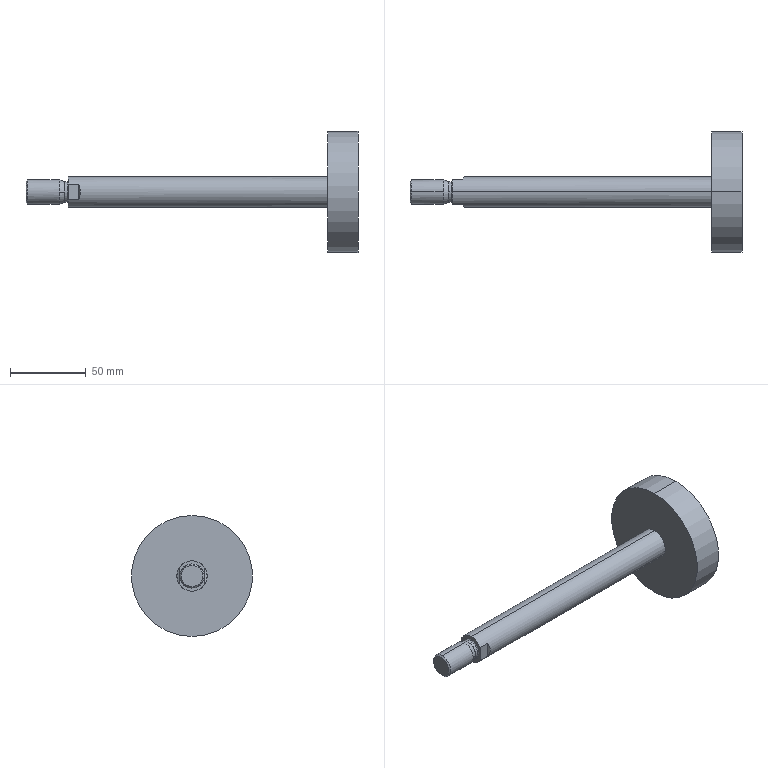Part | SolidWorks | features BaseBody 1 | 1 solid | 24 faces | box 219.5 x 80 x 80 mm | volume 159613 mm3 | cylinder 8 | plane 8 | spline 4 | cone 4 | commonest cylinder face diameters 13.5 x2 16 x2 20 x2 80 x2
STEP:
#1=CARTESIAN_POINT('',(-9.65,0.,6.75));
#2=VERTEX_POINT('',#1);
#3=CARTESIAN_POINT('',(-9.65,0.,-6.75));
#4=VERTEX_POINT('',#3);
#5=CARTESIAN_POINT('',(-9.65,0.,0.));
#6=DIRECTION('',(-1.,0.,0.));
#7=DIRECTION('',(0.,0.,-1.));
#8=AXIS2_PLACEMENT_3D('',#5,#6,#7);
#9=CIRCLE('',#8,6.75);
#10=EDGE_CURVE('',#2,#4,#9,.T.);
#11=ORIENTED_EDGE('',*,*,#10,.F.);
#12=CARTESIAN_POINT('',(-8.9,0.,7.5));
#13=VERTEX_POINT('',#12);
#14=CARTESIAN_POINT('',(-9.65,0.,7.5));
#15=DIRECTION('',(0.,-1.,0.));
#16=DIRECTION('',(0.,0.,1.));
#17=AXIS2_PLACEMENT_3D('',#14,#15,#16);
#18=CIRCLE('',#17,0.75);
#19=EDGE_CURVE('',#2,#13,#18,.T.);
#20=ORIENTED_EDGE('',*,*,#19,.T.);
#21=CARTESIAN_POINT('',(-8.9,0.,-7.5));
#22=VERTEX_POINT('',#21);
#23=CARTESIAN_POINT('',(-8.9,0.,7.5));
#24=CARTESIAN_POINT('',(-8.9,15.,7.5));
#25=CARTESIAN_POINT('',(-8.9,15.,-7.5));
#26=CARTESIAN_POINT('',(-8.9,0.,-7.5));
#27=(BOUNDED_CURVE()B_SPLINE_CURVE(3,(#23,#24,#25,#26),.UNSPECIFIED.,.F.,.T.)B_SPLINE_CURVE_WITH_KNOTS((4,4),(0.5,1.),.UNSPECIFIED.)CURVE()GEOMETRIC_REPRESENTATION_ITEM()RATIONAL_B_SPLINE_CURVE((1.,0.3333,0.3333,1.))REPRESENTATION_ITEM(''));
#28=EDGE_CURVE('',#13,#22,#27,.T.);
#29=ORIENTED_EDGE('',*,*,#28,.T.);
#30=CARTESIAN_POINT('',(-9.65,0.,-7.5));
#31=DIRECTION('',(0.,1.,0.));
#32=DIRECTION('',(0.,0.,-1.));
#33=AXIS2_PLACEMENT_3D('',#30,#31,#32);
#34=CIRCLE('',#33,0.75);
#35=EDGE_CURVE('',#4,#22,#34,.T.);
#36=ORIENTED_EDGE('',*,*,#35,.F.);
#37=EDGE_LOOP('',(#11,#20,#29,#36));
#38=FACE_OUTER_BOUND('',#37,.T.);
#39=CARTESIAN_POINT('',(-9.65,0.,-6.75));
#40=CARTESIAN_POINT('',(-9.65,13.5,-6.75));
#41=CARTESIAN_POINT('',(-9.65,13.5,6.75));
#42=CARTESIAN_POINT('',(-9.65,0.,6.75));
#43=CARTESIAN_POINT('',(-9.211,0.,-6.75));
#44=CARTESIAN_POINT('',(-9.211,13.5,-6.75));
#45=CARTESIAN_POINT('',(-9.211,13.5,6.75));
#46=CARTESIAN_POINT('',(-9.211,0.,6.75));
#47=CARTESIAN_POINT('',(-8.9,0.,-7.061));
#48=CARTESIAN_POINT('',(-8.9,14.121,-7.061));
#49=CARTESIAN_POINT('',(-8.9,14.121,7.061));
#50=CARTESIAN_POINT('',(-8.9,0.,7.061));
#51=CARTESIAN_POINT('',(-8.9,0.,-7.5));
#52=CARTESIAN_POINT('',(-8.9,15.,-7.5));
#53=CARTESIAN_POINT('',(-8.9,15.,7.5));
#54=CARTESIAN_POINT('',(-8.9,0.,7.5));
#55=(BOUNDED_SURFACE()B_SPLINE_SURFACE(3,3,((#39,#40,#41,#42),(#43,#44,#45,#46),(#47,#48,#49,#50),(#51,#52,#53,#54)),.UNSPECIFIED.,.F.,.F.,.T.)B_SPLINE_SURFACE_WITH_KNOTS((4,4),(4,4),(0.,1.),(0.,1.),.UNSPECIFIED.)GEOMETRIC_REPRESENTATION_ITEM()RATIONAL_B_SPLINE_SURFACE(((1.,0.3333,0.3333,1.),(0.8047,0.2682,0.2682,0.8047),(0.8047,0.2682,0.2682,0.8047),(1.,0.3333,0.3333,1.)))REPRESENTATION_ITEM('')SURFACE());
#56=ADVANCED_FACE('',(#38),#55,.F.);
#57=CARTESIAN_POINT('',(-11.624,0.,6.795));
#58=VERTEX_POINT('',#57);
#59=CARTESIAN_POINT('',(-11.624,6.795,0.));
#60=VERTEX_POINT('',#59);
#61=CARTESIAN_POINT('',(-11.624,0.,0.));
#62=DIRECTION('',(-1.,0.,0.));
#63=DIRECTION('',(0.,0.,-1.));
#64=AXIS2_PLACEMENT_3D('',#61,#62,#63);
#65=CIRCLE('',#64,6.795);
#66=EDGE_CURVE('',#58,#60,#65,.T.);
#67=ORIENTED_EDGE('',*,*,#66,.F.);
#68=CARTESIAN_POINT('',(-11.368,0.,6.75));
#69=VERTEX_POINT('',#68);
#70=CARTESIAN_POINT('',(-11.368,0.,7.5));
#71=DIRECTION('',(0.,-1.,0.));
#72=DIRECTION('',(0.,0.,1.));
#73=AXIS2_PLACEMENT_3D('',#70,#71,#72);
#74=CIRCLE('',#73,0.75);
#75=EDGE_CURVE('',#58,#69,#74,.T.);
#76=ORIENTED_EDGE('',*,*,#75,.T.);
#77=CARTESIAN_POINT('',(-11.368,0.,-6.75));
#78=VERTEX_POINT('',#77);
#79=CARTESIAN_POINT('',(-11.368,0.,0.));
#80=DIRECTION('',(1.,0.,0.));
#81=DIRECTION('',(0.,0.,1.));
#82=AXIS2_PLACEMENT_3D('',#79,#80,#81);
#83=CIRCLE('',#82,6.75);
#84=EDGE_CURVE('',#78,#69,#83,.T.);
#85=ORIENTED_EDGE('',*,*,#84,.F.);
#86=CARTESIAN_POINT('',(-11.624,0.,-6.795));
#87=VERTEX_POINT('',#86);
#88=CARTESIAN_POINT('',(-11.368,0.,-7.5));
#89=DIRECTION('',(0.,1.,0.));
#90=DIRECTION('',(0.,0.,-1.));
#91=AXIS2_PLACEMENT_3D('',#88,#89,#90);
#92=CIRCLE('',#91,0.75);
#93=EDGE_CURVE('',#87,#78,#92,.T.);
#94=ORIENTED_EDGE('',*,*,#93,.F.);
#95=CARTESIAN_POINT('',(-11.624,0.,0.));
#96=DIRECTION('',(-1.,0.,0.));
#97=DIRECTION('',(0.,0.,-1.));
#98=AXIS2_PLACEMENT_3D('',#95,#96,#97);
#99=CIRCLE('',#98,6.795);
#100=EDGE_CURVE('',#60,#87,#99,.T.);
#101=ORIENTED_EDGE('',*,*,#100,.F.);
#102=EDGE_LOOP('',(#67,#76,#85,#94,#101));
#103=FACE_OUTER_BOUND('',#102,.T.);
#104=CARTESIAN_POINT('',(-11.624,0.,-6.795));
#105=CARTESIAN_POINT('',(-11.624,13.59,-6.795));
#106=CARTESIAN_POINT('',(-11.624,13.59,6.795));
#107=CARTESIAN_POINT('',(-11.624,0.,6.795));
#108=CARTESIAN_POINT('',(-11.542,0.,-6.765));
#109=CARTESIAN_POINT('',(-11.542,13.53,-6.765));
#110=CARTESIAN_POINT('',(-11.542,13.53,6.765));
#111=CARTESIAN_POINT('',(-11.542,0.,6.765));
#112=CARTESIAN_POINT('',(-11.455,0.,-6.75));
#113=CARTESIAN_POINT('',(-11.455,13.5,-6.75));
#114=CARTESIAN_POINT('',(-11.455,13.5,6.75));
#115=CARTESIAN_POINT('',(-11.455,0.,6.75));
#116=CARTESIAN_POINT('',(-11.368,0.,-6.75));
#117=CARTESIAN_POINT('',(-11.368,13.5,-6.75));
#118=CARTESIAN_POINT('',(-11.368,13.5,6.75));
#119=CARTESIAN_POINT('',(-11.368,0.,6.75));
#120=(BOUNDED_SURFACE()B_SPLINE_SURFACE(3,3,((#104,#105,#106,#107),(#108,#109,#110,#111),(#112,#113,#114,#115),(#116,#117,#118,#119)),.UNSPECIFIED.,.F.,.F.,.F.)B_SPLINE_SURFACE_WITH_KNOTS((4,4),(4,4),(0.,1.),(0.,1.),.UNSPECIFIED.)GEOMETRIC_REPRESENTATION_ITEM()RATIONAL_B_SPLINE_SURFACE(((1.,0.3333,0.3333,1.),(0.9899,0.33,0.33,0.9899),(0.9899,0.33,0.33,0.9899),(1.,0.3333,0.3333,1.)))REPRESENTATION_ITEM('')SURFACE());
#121=ADVANCED_FACE('',(#103),#120,.F.);
#122=CARTESIAN_POINT('',(162.6,0.,10.));
#123=VERTEX_POINT('',#122);
#124=CARTESIAN_POINT('',(162.6,0.,-10.));
#125=VERTEX_POINT('',#124);
#126=CARTESIAN_POINT('',(162.6,0.,0.));
#127=DIRECTION('',(-1.,0.,0.));
#128=DIRECTION('',(0.,0.,1.));
#129=AXIS2_PLACEMENT_3D('',#126,#127,#128);
#130=CIRCLE('',#129,10.);
#131=EDGE_CURVE('',#123,#125,#130,.T.);
#132=ORIENTED_EDGE('',*,*,#131,.T.);
#133=CARTESIAN_POINT('',(-8.9,0.,-10.));
#134=VERTEX_POINT('',#133);
#135=CARTESIAN_POINT('',(182.6,0.,-10.));
#136=DIRECTION('',(-1.,0.,0.));
#137=VECTOR('',#136,1000.);
#138=LINE('',#135,#137);
#139=EDGE_CURVE('',#125,#134,#138,.T.);
#140=ORIENTED_EDGE('',*,*,#139,.T.);
#141=CARTESIAN_POINT('',(-8.9,8.5,-5.268));
#142=VERTEX_POINT('',#141);
#143=CARTESIAN_POINT('',(-8.9,0.,0.));
#144=DIRECTION('',(1.,0.,0.));
#145=DIRECTION('',(0.,0.,1.));
#146=AXIS2_PLACEMENT_3D('',#143,#144,#145);
#147=CIRCLE('',#146,10.);
#148=EDGE_CURVE('',#134,#142,#147,.T.);
#149=ORIENTED_EDGE('',*,*,#148,.T.);
#150=CARTESIAN_POINT('',(-1.9,8.5,-5.268));
#151=VERTEX_POINT('',#150);
#152=CARTESIAN_POINT('',(182.6,8.5,-5.268));
#153=DIRECTION('',(1.,0.,0.));
#154=VECTOR('',#153,1000.);
#155=LINE('',#152,#154);
#156=EDGE_CURVE('',#142,#151,#155,.T.);
#157=ORIENTED_EDGE('',*,*,#156,.T.);
#158=CARTESIAN_POINT('',(-1.9,8.5,5.268));
#159=VERTEX_POINT('',#158);
#160=CARTESIAN_POINT('',(-1.9,8.5,-5.268));
#161=CARTESIAN_POINT('',(-0.7132,10.556,-1.951));
#162=CARTESIAN_POINT('',(-0.7132,10.556,1.951));
#163=CARTESIAN_POINT('',(-1.9,8.5,5.268));
#164=(BOUNDED_CURVE()B_SPLINE_CURVE(3,(#160,#161,#162,#163),.UNSPECIFIED.,.F.,.F.)B_SPLINE_CURVE_WITH_KNOTS((4,4),(2.587,3.696),.UNSPECIFIED.)CURVE()GEOMETRIC_REPRESENTATION_ITEM()RATIONAL_B_SPLINE_CURVE((1.,0.9,0.9,1.))REPRESENTATION_ITEM(''));
#165=EDGE_CURVE('',#151,#159,#164,.T.);
#166=ORIENTED_EDGE('',*,*,#165,.T.);
#167=CARTESIAN_POINT('',(-8.9,8.5,5.268));
#168=VERTEX_POINT('',#167);
#169=CARTESIAN_POINT('',(182.6,8.5,5.268));
#170=DIRECTION('',(-1.,0.,0.));
#171=VECTOR('',#170,1000.);
#172=LINE('',#169,#171);
#173=EDGE_CURVE('',#159,#168,#172,.T.);
#174=ORIENTED_EDGE('',*,*,#173,.T.);
#175=CARTESIAN_POINT('',(-8.9,0.,10.));
#176=VERTEX_POINT('',#175);
#177=CARTESIAN_POINT('',(-8.9,0.,0.));
#178=DIRECTION('',(1.,0.,0.));
#179=DIRECTION('',(0.,0.,1.));
#180=AXIS2_PLACEMENT_3D('',#177,#178,#179);
#181=CIRCLE('',#180,10.);
#182=EDGE_CURVE('',#168,#176,#181,.T.);
#183=ORIENTED_EDGE('',*,*,#182,.T.);
#184=CARTESIAN_POINT('',(182.6,0.,10.));
#185=DIRECTION('',(-1.,0.,0.));
#186=VECTOR('',#185,1000.);
#187=LINE('',#184,#186);
#188=EDGE_CURVE('',#123,#176,#187,.T.);
#189=ORIENTED_EDGE('',*,*,#188,.F.);
#190=EDGE_LOOP('',(#132,#140,#149,#157,#166,#174,#183,#189));
#191=FACE_OUTER_BOUND('',#190,.T.);
#192=CARTESIAN_POINT('',(182.6,0.,0.));
#193=DIRECTION('',(-1.,0.,0.));
#194=DIRECTION('',(0.,0.,1.));
#195=AXIS2_PLACEMENT_3D('',#192,#193,#194);
#196=CYLINDRICAL_SURFACE('',#195,10.);
#197=ADVANCED_FACE('',(#191),#196,.T.);
#198=CARTESIAN_POINT('',(182.6,0.,40.));
#199=VERTEX_POINT('',#198);
#200=CARTESIAN_POINT('',(182.6,0.,-40.));
#201=VERTEX_POINT('',#200);
#202=CARTESIAN_POINT('',(182.6,0.,0.));
#203=DIRECTION('',(-1.,0.,0.));
#204=DIRECTION('',(0.,0.,1.));
#205=AXIS2_PLACEMENT_3D('',#202,#203,#204);
#206=CIRCLE('',#205,40.);
#207=EDGE_CURVE('',#199,#201,#206,.T.);
#208=ORIENTED_EDGE('',*,*,#207,.T.);
#209=CARTESIAN_POINT('',(162.6,0.,-40.));
#210=VERTEX_POINT('',#209);
#211=CARTESIAN_POINT('',(182.6,0.,-40.));
#212=DIRECTION('',(-1.,0.,0.));
#213=VECTOR('',#212,1000.);
#214=LINE('',#211,#213);
#215=EDGE_CURVE('',#201,#210,#214,.T.);
#216=ORIENTED_EDGE('',*,*,#215,.T.);
#217=CARTESIAN_POINT('',(162.6,0.,40.));
#218=VERTEX_POINT('',#217);
#219=CARTESIAN_POINT('',(162.6,0.,0.));
#220=DIRECTION('',(1.,0.,0.));
#221=DIRECTION('',(0.,0.,1.));
#222=AXIS2_PLACEMENT_3D('',#219,#220,#221);
#223=CIRCLE('',#222,40.);
#224=EDGE_CURVE('',#210,#218,#223,.T.);
#225=ORIENTED_EDGE('',*,*,#224,.T.);
#226=CARTESIAN_POINT('',(182.6,0.,40.));
#227=DIRECTION('',(-1.,0.,0.));
#228=VECTOR('',#227,1000.);
#229=LINE('',#226,#228);
#230=EDGE_CURVE('',#199,#218,#229,.T.);
#231=ORIENTED_EDGE('',*,*,#230,.F.);
#232=EDGE_LOOP('',(#208,#216,#225,#231));
#233=FACE_OUTER_BOUND('',#232,.T.);
#234=CARTESIAN_POINT('',(182.6,0.,0.));
#235=DIRECTION('',(-1.,0.,0.));
#236=DIRECTION('',(0.,0.,1.));
#237=AXIS2_PLACEMENT_3D('',#234,#235,#236);
#238=CYLINDRICAL_SURFACE('',#237,40.);
#239=ADVANCED_FACE('',(#233),#238,.T.);
#240=ORIENTED_EDGE('',*,*,#10,.T.);
#241=CARTESIAN_POINT('',(-7.9,0.,-6.75));
#242=DIRECTION('',(-1.,0.,0.));
#243=VECTOR('',#242,1000.);
#244=LINE('',#241,#243);
#245=EDGE_CURVE('',#4,#78,#244,.T.);
#246=ORIENTED_EDGE('',*,*,#245,.T.);
#247=ORIENTED_EDGE('',*,*,#84,.T.);
#248=CARTESIAN_POINT('',(-7.9,0.,6.75));
#249=DIRECTION('',(-1.,0.,0.));
#250=VECTOR('',#249,1000.);
#251=LINE('',#248,#250);
#252=EDGE_CURVE('',#2,#69,#251,.T.);
#253=ORIENTED_EDGE('',*,*,#252,.F.);
#254=EDGE_LOOP('',(#240,#246,#247,#253));
#255=FACE_OUTER_BOUND('',#254,.T.);
#256=CARTESIAN_POINT('',(-7.9,0.,0.));
#257=DIRECTION('',(-1.,0.,0.));
#258=DIRECTION('',(0.,0.,1.));
#259=AXIS2_PLACEMENT_3D('',#256,#257,#258);
#260=CYLINDRICAL_SURFACE('',#259,6.75);
#261=ADVANCED_FACE('',(#255),#260,.T.);
#262=CARTESIAN_POINT('',(-11.624,-6.795,0.));
#263=VERTEX_POINT('',#262);
#264=CARTESIAN_POINT('',(-11.624,0.,0.));
#265=DIRECTION('',(-1.,0.,0.));
#266=DIRECTION('',(0.,0.,-1.));
#267=AXIS2_PLACEMENT_3D('',#264,#265,#266);
#268=CIRCLE('',#267,6.795);
#269=EDGE_CURVE('',#263,#58,#268,.T.);
#270=ORIENTED_EDGE('',*,*,#269,.T.);
#271=ORIENTED_EDGE('',*,*,#66,.T.);
#272=CARTESIAN_POINT('',(-14.934,8.,0.));
#273=VERTEX_POINT('',#272);
#274=CARTESIAN_POINT('',(-14.934,8.,0.));
#275=DIRECTION('',(-0.9397,0.342,0.));
#276=VECTOR('',#275,1000.);
#277=LINE('',#274,#276);
#278=EDGE_CURVE('',#60,#273,#277,.T.);
#279=ORIENTED_EDGE('',*,*,#278,.T.);
#280=CARTESIAN_POINT('',(-14.934,0.,8.));
#281=VERTEX_POINT('',#280);
#282=CARTESIAN_POINT('',(-14.934,0.,0.));
#283=DIRECTION('',(1.,0.,0.));
#284=DIRECTION('',(0.,0.,1.));
#285=AXIS2_PLACEMENT_3D('',#282,#283,#284);
#286=CIRCLE('',#285,8.);
#287=EDGE_CURVE('',#273,#281,#286,.T.);
#288=ORIENTED_EDGE('',*,*,#287,.T.);
#289=CARTESIAN_POINT('',(-14.934,-8.,0.));
#290=VERTEX_POINT('',#289);
#291=CARTESIAN_POINT('',(-14.934,0.,0.));
#292=DIRECTION('',(1.,0.,0.));
#293=DIRECTION('',(0.,0.,1.));
#294=AXIS2_PLACEMENT_3D('',#291,#292,#293);
#295=CIRCLE('',#294,8.);
#296=EDGE_CURVE('',#281,#290,#295,.T.);
#297=ORIENTED_EDGE('',*,*,#296,.T.);
#298=CARTESIAN_POINT('',(-14.934,-8.,0.));
#299=DIRECTION('',(-0.9397,-0.342,0.));
#300=VECTOR('',#299,1000.);
#301=LINE('',#298,#300);
#302=EDGE_CURVE('',#263,#290,#301,.T.);
#303=ORIENTED_EDGE('',*,*,#302,.F.);
#304=EDGE_LOOP('',(#270,#271,#279,#288,#297,#303));
#305=FACE_OUTER_BOUND('',#304,.T.);
#306=CARTESIAN_POINT('',(-14.934,0.,0.));
#307=DIRECTION('',(-1.,0.,0.));
#308=DIRECTION('',(0.,-1.,0.));
#309=AXIS2_PLACEMENT_3D('',#306,#307,#308);
#310=CONICAL_SURFACE('',#309,8.,0.3491);
#311=ADVANCED_FACE('',(#305),#310,.T.);
#312=CARTESIAN_POINT('',(-14.934,0.,-8.));
#313=VERTEX_POINT('',#312);
#314=CARTESIAN_POINT('',(-14.934,0.,0.));
#315=DIRECTION('',(1.,0.,0.));
#316=DIRECTION('',(0.,0.,1.));
#317=AXIS2_PLACEMENT_3D('',#314,#315,#316);
#318=CIRCLE('',#317,8.);
#319=EDGE_CURVE('',#313,#273,#318,.T.);
#320=ORIENTED_EDGE('',*,*,#319,.F.);
#321=CARTESIAN_POINT('',(-35.98,0.,-8.));
#322=VERTEX_POINT('',#321);
#323=CARTESIAN_POINT('',(-7.9,0.,-8.));
#324=DIRECTION('',(-1.,0.,0.));
#325=VECTOR('',#324,1000.);
#326=LINE('',#323,#325);
#327=EDGE_CURVE('',#313,#322,#326,.T.);
#328=ORIENTED_EDGE('',*,*,#327,.T.);
#329=CARTESIAN_POINT('',(-35.98,0.,8.));
#330=VERTEX_POINT('',#329);
#331=CARTESIAN_POINT('',(-35.98,0.,0.));
#332=DIRECTION('',(1.,0.,0.));
#333=DIRECTION('',(0.,0.,1.));
#334=AXIS2_PLACEMENT_3D('',#331,#332,#333);
#335=CIRCLE('',#334,8.);
#336=EDGE_CURVE('',#322,#330,#335,.T.);
#337=ORIENTED_EDGE('',*,*,#336,.T.);
#338=CARTESIAN_POINT('',(-7.9,0.,8.));
#339=DIRECTION('',(-1.,0.,0.));
#340=VECTOR('',#339,1000.);
#341=LINE('',#338,#340);
#342=EDGE_CURVE('',#281,#330,#341,.T.);
#343=ORIENTED_EDGE('',*,*,#342,.F.);
#344=ORIENTED_EDGE('',*,*,#287,.F.);
#345=EDGE_LOOP('',(#320,#328,#337,#343,#344));
#346=FACE_OUTER_BOUND('',#345,.T.);
#347=CARTESIAN_POINT('',(-7.9,0.,0.));
#348=DIRECTION('',(-1.,0.,0.));
#349=DIRECTION('',(0.,0.,1.));
#350=AXIS2_PLACEMENT_3D('',#347,#348,#349);
#351=CYLINDRICAL_SURFACE('',#350,8.);
#352=ADVANCED_FACE('',(#346),#351,.T.);
#353=CARTESIAN_POINT('',(-36.9,0.,-7.08));
#354=VERTEX_POINT('',#353);
#355=CARTESIAN_POINT('',(-36.9,0.,7.08));
#356=VERTEX_POINT('',#355);
#357=CARTESIAN_POINT('',(-36.9,0.,0.));
#358=DIRECTION('',(1.,0.,0.));
#359=DIRECTION('',(0.,0.,-1.));
#360=AXIS2_PLACEMENT_3D('',#357,#358,#359);
#361=CIRCLE('',#360,7.08);
#362=EDGE_CURVE('',#354,#356,#361,.T.);
#363=ORIENTED_EDGE('',*,*,#362,.T.);
#364=CARTESIAN_POINT('',(-35.98,0.,8.));
#365=DIRECTION('',(0.7071,0.,0.7071));
#366=VECTOR('',#365,1000.);
#367=LINE('',#364,#366);
#368=EDGE_CURVE('',#356,#330,#367,.T.);
#369=ORIENTED_EDGE('',*,*,#368,.T.);
#370=ORIENTED_EDGE('',*,*,#336,.F.);
#371=CARTESIAN_POINT('',(-35.98,0.,-8.));
#372=DIRECTION('',(0.7071,0.,-0.7071));
#373=VECTOR('',#372,1000.);
#374=LINE('',#371,#373);
#375=EDGE_CURVE('',#354,#322,#374,.T.);
#376=ORIENTED_EDGE('',*,*,#375,.F.);
#377=EDGE_LOOP('',(#363,#369,#370,#376));
#378=FACE_OUTER_BOUND('',#377,.T.);
#379=CARTESIAN_POINT('',(-35.98,0.,0.));
#380=DIRECTION('',(1.,0.,0.));
#381=DIRECTION('',(0.,0.,-1.));
#382=AXIS2_PLACEMENT_3D('',#379,#380,#381);
#383=CONICAL_SURFACE('',#382,8.,0.7854);
#384=ADVANCED_FACE('',(#378),#383,.T.);
#385=ORIENTED_EDGE('',*,*,#139,.F.);
#386=CARTESIAN_POINT('',(162.6,0.,0.));
#387=DIRECTION('',(-1.,0.,0.));
#388=DIRECTION('',(0.,0.,1.));
#389=AXIS2_PLACEMENT_3D('',#386,#387,#388);
#390=CIRCLE('',#389,10.);
#391=EDGE_CURVE('',#125,#123,#390,.T.);
#392=ORIENTED_EDGE('',*,*,#391,.T.);
#393=ORIENTED_EDGE('',*,*,#188,.T.);
#394=CARTESIAN_POINT('',(-8.9,-8.5,5.268));
#395=VERTEX_POINT('',#394);
#396=CARTESIAN_POINT('',(-8.9,0.,0.));
#397=DIRECTION('',(1.,0.,0.));
#398=DIRECTION('',(0.,0.,1.));
#399=AXIS2_PLACEMENT_3D('',#396,#397,#398);
#400=CIRCLE('',#399,10.);
#401=EDGE_CURVE('',#176,#395,#400,.T.);
#402=ORIENTED_EDGE('',*,*,#401,.T.);
#403=CARTESIAN_POINT('',(-1.9,-8.5,5.268));
#404=VERTEX_POINT('',#403);
#405=CARTESIAN_POINT('',(182.6,-8.5,5.268));
#406=DIRECTION('',(1.,0.,0.));
#407=VECTOR('',#406,1000.);
#408=LINE('',#405,#407);
#409=EDGE_CURVE('',#395,#404,#408,.T.);
#410=ORIENTED_EDGE('',*,*,#409,.T.);
#411=CARTESIAN_POINT('',(-1.9,-8.5,-5.268));
#412=VERTEX_POINT('',#411);
#413=CARTESIAN_POINT('',(-1.9,-8.5,5.268));
#414=CARTESIAN_POINT('',(-0.7132,-10.556,1.951));
#415=CARTESIAN_POINT('',(-0.7132,-10.556,-1.951));
#416=CARTESIAN_POINT('',(-1.9,-8.5,-5.268));
#417=(BOUNDED_CURVE()B_SPLINE_CURVE(3,(#413,#414,#415,#416),.UNSPECIFIED.,.F.,.T.)B_SPLINE_CURVE_WITH_KNOTS((4,4),(2.587,3.696),.UNSPECIFIED.)CURVE()GEOMETRIC_REPRESENTATION_ITEM()RATIONAL_B_SPLINE_CURVE((1.,0.9,0.9,1.))REPRESENTATION_ITEM(''));
#418=EDGE_CURVE('',#404,#412,#417,.T.);
#419=ORIENTED_EDGE('',*,*,#418,.T.);
#420=CARTESIAN_POINT('',(-8.9,-8.5,-5.268));
#421=VERTEX_POINT('',#420);
#422=CARTESIAN_POINT('',(182.6,-8.5,-5.268));
#423=DIRECTION('',(-1.,0.,0.));
#424=VECTOR('',#423,1000.);
#425=LINE('',#422,#424);
#426=EDGE_CURVE('',#412,#421,#425,.T.);
#427=ORIENTED_EDGE('',*,*,#426,.T.);
#428=CARTESIAN_POINT('',(-8.9,0.,0.));
#429=DIRECTION('',(1.,0.,0.));
#430=DIRECTION('',(0.,0.,1.));
#431=AXIS2_PLACEMENT_3D('',#428,#429,#430);
#432=CIRCLE('',#431,10.);
#433=EDGE_CURVE('',#421,#134,#432,.T.);
#434=ORIENTED_EDGE('',*,*,#433,.T.);
#435=EDGE_LOOP('',(#385,#392,#393,#402,#410,#419,#427,#434));
#436=FACE_OUTER_BOUND('',#435,.T.);
#437=CARTESIAN_POINT('',(182.6,0.,0.));
#438=DIRECTION('',(-1.,0.,0.));
#439=DIRECTION('',(0.,0.,1.));
#440=AXIS2_PLACEMENT_3D('',#437,#438,#439);
#441=CYLINDRICAL_SURFACE('',#440,10.);
#442=ADVANCED_FACE('',(#436),#441,.T.);
#443=ORIENTED_EDGE('',*,*,#418,.F.);
#444=CARTESIAN_POINT('',(-1.9,-8.5,20.));
#445=DIRECTION('',(0.,0.,-1.));
#446=VECTOR('',#445,1000.);
#447=LINE('',#444,#446);
#448=EDGE_CURVE('',#404,#412,#447,.T.);
#449=ORIENTED_EDGE('',*,*,#448,.T.);
#450=EDGE_LOOP('',(#443,#449));
#451=FACE_OUTER_BOUND('',#450,.T.);
#452=CARTESIAN_POINT('',(6.76,-23.5,20.));
#453=DIRECTION('',(-0.866,-0.5,0.));
#454=DIRECTION('',(0.5,-0.866,0.));
#455=AXIS2_PLACEMENT_3D('',#452,#453,#454);
#456=PLANE('',#455);
#457=ADVANCED_FACE('',(#451),#456,.T.);
#458=ORIENTED_EDGE('',*,*,#409,.F.);
#459=CARTESIAN_POINT('',(-8.9,-8.5,20.));
#460=DIRECTION('',(0.,0.,-1.));
#461=VECTOR('',#460,1000.);
#462=LINE('',#459,#461);
#463=EDGE_CURVE('',#395,#421,#462,.T.);
#464=ORIENTED_EDGE('',*,*,#463,.T.);
#465=ORIENTED_EDGE('',*,*,#426,.F.);
#466=ORIENTED_EDGE('',*,*,#448,.F.);
#467=EDGE_LOOP('',(#458,#464,#465,#466));
#468=FACE_OUTER_BOUND('',#467,.T.);
#469=CARTESIAN_POINT('',(-1.9,-8.5,20.));
#470=DIRECTION('',(0.,-1.,0.));
#471=DIRECTION('',(0.,0.,-1.));
#472=AXIS2_PLACEMENT_3D('',#469,#470,#471);
#473=PLANE('',#472);
#474=ADVANCED_FACE('',(#468),#473,.T.);
#475=CARTESIAN_POINT('',(-8.9,0.,-7.5));
#476=CARTESIAN_POINT('',(-8.9,-15.,-7.5));
#477=CARTESIAN_POINT('',(-8.9,-15.,7.5));
#478=CARTESIAN_POINT('',(-8.9,0.,7.5));
#479=(BOUNDED_CURVE()B_SPLINE_CURVE(3,(#475,#476,#477,#478),.UNSPECIFIED.,.F.,.T.)B_SPLINE_CURVE_WITH_KNOTS((4,4),(0.,0.5),.UNSPECIFIED.)CURVE()GEOMETRIC_REPRESENTATION_ITEM()RATIONAL_B_SPLINE_CURVE((1.,0.3333,0.3333,1.))REPRESENTATION_ITEM(''));
#480=EDGE_CURVE('',#22,#13,#479,.T.);
#481=ORIENTED_EDGE('',*,*,#480,.F.);
#482=ORIENTED_EDGE('',*,*,#28,.F.);
#483=EDGE_LOOP('',(#481,#482));
#484=FACE_BOUND('',#483,.T.);
#485=ORIENTED_EDGE('',*,*,#433,.F.);
#486=ORIENTED_EDGE('',*,*,#463,.F.);
#487=ORIENTED_EDGE('',*,*,#401,.F.);
#488=ORIENTED_EDGE('',*,*,#182,.F.);
#489=CARTESIAN_POINT('',(-8.9,8.5,0.));
#490=DIRECTION('',(0.,0.,1.));
#491=VECTOR('',#490,1000.);
#492=LINE('',#489,#491);
#493=EDGE_CURVE('',#142,#168,#492,.T.);
#494=ORIENTED_EDGE('',*,*,#493,.F.);
#495=ORIENTED_EDGE('',*,*,#148,.F.);
#496=EDGE_LOOP('',(#485,#486,#487,#488,#494,#495));
#497=FACE_OUTER_BOUND('',#496,.T.);
#498=CARTESIAN_POINT('',(-8.9,0.,0.));
#499=DIRECTION('',(1.,0.,0.));
#500=DIRECTION('',(0.,0.,-1.));
#501=AXIS2_PLACEMENT_3D('',#498,#499,#500);
#502=PLANE('',#501);
#503=ADVANCED_FACE('',(#484,#497),#502,.F.);
#504=ORIENTED_EDGE('',*,*,#156,.F.);
#505=ORIENTED_EDGE('',*,*,#493,.T.);
#506=ORIENTED_EDGE('',*,*,#173,.F.);
#507=CARTESIAN_POINT('',(-1.9,8.5,20.));
#508=DIRECTION('',(0.,0.,-1.));
#509=VECTOR('',#508,1000.);
#510=LINE('',#507,#509);
#511=EDGE_CURVE('',#159,#151,#510,.T.);
#512=ORIENTED_EDGE('',*,*,#511,.T.);
#513=EDGE_LOOP('',(#504,#505,#506,#512));
#514=FACE_OUTER_BOUND('',#513,.T.);
#515=CARTESIAN_POINT('',(-8.9,8.5,20.));
#516=DIRECTION('',(0.,1.,0.));
#517=DIRECTION('',(0.,0.,1.));
#518=AXIS2_PLACEMENT_3D('',#515,#516,#517);
#519=PLANE('',#518);
#520=ADVANCED_FACE('',(#514),#519,.T.);
#521=ORIENTED_EDGE('',*,*,#165,.F.);
#522=ORIENTED_EDGE('',*,*,#511,.F.);
#523=EDGE_LOOP('',(#521,#522));
#524=FACE_OUTER_BOUND('',#523,.T.);
#525=CARTESIAN_POINT('',(-1.9,8.5,20.));
#526=DIRECTION('',(-0.866,0.5,0.));
#527=DIRECTION('',(-0.5,-0.866,0.));
#528=AXIS2_PLACEMENT_3D('',#525,#526,#527);
#529=PLANE('',#528);
#530=ADVANCED_FACE('',(#524),#529,.T.);
#531=ORIENTED_EDGE('',*,*,#131,.F.);
#532=ORIENTED_EDGE('',*,*,#391,.F.);
#533=EDGE_LOOP('',(#531,#532));
#534=FACE_BOUND('',#533,.T.);
#535=CARTESIAN_POINT('',(162.6,0.,0.));
#536=DIRECTION('',(1.,0.,0.));
#537=DIRECTION('',(0.,0.,1.));
#538=AXIS2_PLACEMENT_3D('',#535,#536,#537);
#539=CIRCLE('',#538,40.);
#540=EDGE_CURVE('',#218,#210,#539,.T.);
#541=ORIENTED_EDGE('',*,*,#540,.F.);
#542=ORIENTED_EDGE('',*,*,#224,.F.);
#543=EDGE_LOOP('',(#541,#542));
#544=FACE_OUTER_BOUND('',#543,.T.);
#545=CARTESIAN_POINT('',(162.6,0.,0.));
#546=DIRECTION('',(1.,0.,0.));
#547=DIRECTION('',(0.,0.,-1.));
#548=AXIS2_PLACEMENT_3D('',#545,#546,#547);
#549=PLANE('',#548);
#550=ADVANCED_FACE('',(#534,#544),#549,.F.);
#551=ORIENTED_EDGE('',*,*,#19,.F.);
#552=CARTESIAN_POINT('',(-9.65,0.,0.));
#553=DIRECTION('',(-1.,0.,0.));
#554=DIRECTION('',(0.,0.,-1.));
#555=AXIS2_PLACEMENT_3D('',#552,#553,#554);
#556=CIRCLE('',#555,6.75);
#557=EDGE_CURVE('',#4,#2,#556,.T.);
#558=ORIENTED_EDGE('',*,*,#557,.F.);
#559=ORIENTED_EDGE('',*,*,#35,.T.);
#560=ORIENTED_EDGE('',*,*,#480,.T.);
#561=EDGE_LOOP('',(#551,#558,#559,#560));
#562=FACE_OUTER_BOUND('',#561,.T.);
#563=CARTESIAN_POINT('',(-9.65,0.,6.75));
#564=CARTESIAN_POINT('',(-9.65,-13.5,6.75));
#565=CARTESIAN_POINT('',(-9.65,-13.5,-6.75));
#566=CARTESIAN_POINT('',(-9.65,0.,-6.75));
#567=CARTESIAN_POINT('',(-9.211,0.,6.75));
#568=CARTESIAN_POINT('',(-9.211,-13.5,6.75));
#569=CARTESIAN_POINT('',(-9.211,-13.5,-6.75));
#570=CARTESIAN_POINT('',(-9.211,0.,-6.75));
#571=CARTESIAN_POINT('',(-8.9,0.,7.061));
#572=CARTESIAN_POINT('',(-8.9,-14.121,7.061));
#573=CARTESIAN_POINT('',(-8.9,-14.121,-7.061));
#574=CARTESIAN_POINT('',(-8.9,0.,-7.061));
#575=CARTESIAN_POINT('',(-8.9,0.,7.5));
#576=CARTESIAN_POINT('',(-8.9,-15.,7.5));
#577=CARTESIAN_POINT('',(-8.9,-15.,-7.5));
#578=CARTESIAN_POINT('',(-8.9,0.,-7.5));
#579=(BOUNDED_SURFACE()B_SPLINE_SURFACE(3,3,((#563,#564,#565,#566),(#567,#568,#569,#570),(#571,#572,#573,#574),(#575,#576,#577,#578)),.UNSPECIFIED.,.F.,.F.,.F.)B_SPLINE_SURFACE_WITH_KNOTS((4,4),(4,4),(0.,1.),(0.,1.),.UNSPECIFIED.)GEOMETRIC_REPRESENTATION_ITEM()RATIONAL_B_SPLINE_SURFACE(((1.,0.3333,0.3333,1.),(0.8047,0.2682,0.2682,0.8047),(0.8047,0.2682,0.2682,0.8047),(1.,0.3333,0.3333,1.)))REPRESENTATION_ITEM('')SURFACE());
#580=ADVANCED_FACE('',(#562),#579,.F.);
#581=ORIENTED_EDGE('',*,*,#215,.F.);
#582=CARTESIAN_POINT('',(182.6,0.,0.));
#583=DIRECTION('',(-1.,0.,0.));
#584=DIRECTION('',(0.,0.,1.));
#585=AXIS2_PLACEMENT_3D('',#582,#583,#584);
#586=CIRCLE('',#585,40.);
#587=EDGE_CURVE('',#201,#199,#586,.T.);
#588=ORIENTED_EDGE('',*,*,#587,.T.);
#589=ORIENTED_EDGE('',*,*,#230,.T.);
#590=ORIENTED_EDGE('',*,*,#540,.T.);
#591=EDGE_LOOP('',(#581,#588,#589,#590));
#592=FACE_OUTER_BOUND('',#591,.T.);
#593=CARTESIAN_POINT('',(182.6,0.,0.));
#594=DIRECTION('',(-1.,0.,0.));
#595=DIRECTION('',(0.,0.,1.));
#596=AXIS2_PLACEMENT_3D('',#593,#594,#595);
#597=CYLINDRICAL_SURFACE('',#596,40.);
#598=ADVANCED_FACE('',(#592),#597,.T.);
#599=ORIENTED_EDGE('',*,*,#245,.F.);
#600=ORIENTED_EDGE('',*,*,#557,.T.);
#601=ORIENTED_EDGE('',*,*,#252,.T.);
#602=CARTESIAN_POINT('',(-11.368,0.,0.));
#603=DIRECTION('',(1.,0.,0.));
#604=DIRECTION('',(0.,0.,1.));
#605=AXIS2_PLACEMENT_3D('',#602,#603,#604);
#606=CIRCLE('',#605,6.75);
#607=EDGE_CURVE('',#69,#78,#606,.T.);
#608=ORIENTED_EDGE('',*,*,#607,.T.);
#609=EDGE_LOOP('',(#599,#600,#601,#608));
#610=FACE_OUTER_BOUND('',#609,.T.);
#611=CARTESIAN_POINT('',(-7.9,0.,0.));
#612=DIRECTION('',(-1.,0.,0.));
#613=DIRECTION('',(0.,0.,1.));
#614=AXIS2_PLACEMENT_3D('',#611,#612,#613);
#615=CYLINDRICAL_SURFACE('',#614,6.75);
#616=ADVANCED_FACE('',(#610),#615,.T.);
#617=ORIENTED_EDGE('',*,*,#207,.F.);
#618=ORIENTED_EDGE('',*,*,#587,.F.);
#619=EDGE_LOOP('',(#617,#618));
#620=FACE_OUTER_BOUND('',#619,.T.);
#621=CARTESIAN_POINT('',(182.6,10.,0.));
#622=DIRECTION('',(-1.,0.,0.));
#623=DIRECTION('',(0.,0.,1.));
#624=AXIS2_PLACEMENT_3D('',#621,#622,#623);
#625=PLANE('',#624);
#626=ADVANCED_FACE('',(#620),#625,.F.);
#627=ORIENTED_EDGE('',*,*,#75,.F.);
#628=ORIENTED_EDGE('',*,*,#269,.F.);
#629=CARTESIAN_POINT('',(-11.624,0.,0.));
#630=DIRECTION('',(-1.,0.,0.));
#631=DIRECTION('',(0.,0.,-1.));
#632=AXIS2_PLACEMENT_3D('',#629,#630,#631);
#633=CIRCLE('',#632,6.795);
#634=EDGE_CURVE('',#87,#263,#633,.T.);
#635=ORIENTED_EDGE('',*,*,#634,.F.);
#636=ORIENTED_EDGE('',*,*,#93,.T.);
#637=ORIENTED_EDGE('',*,*,#607,.F.);
#638=EDGE_LOOP('',(#627,#628,#635,#636,#637));
#639=FACE_OUTER_BOUND('',#638,.T.);
#640=CARTESIAN_POINT('',(-11.624,0.,6.795));
#641=CARTESIAN_POINT('',(-11.624,-13.59,6.795));
#642=CARTESIAN_POINT('',(-11.624,-13.59,-6.795));
#643=CARTESIAN_POINT('',(-11.624,0.,-6.795));
#644=CARTESIAN_POINT('',(-11.542,0.,6.765));
#645=CARTESIAN_POINT('',(-11.542,-13.53,6.765));
#646=CARTESIAN_POINT('',(-11.542,-13.53,-6.765));
#647=CARTESIAN_POINT('',(-11.542,0.,-6.765));
#648=CARTESIAN_POINT('',(-11.455,0.,6.75));
#649=CARTESIAN_POINT('',(-11.455,-13.5,6.75));
#650=CARTESIAN_POINT('',(-11.455,-13.5,-6.75));
#651=CARTESIAN_POINT('',(-11.455,0.,-6.75));
#652=CARTESIAN_POINT('',(-11.368,0.,6.75));
#653=CARTESIAN_POINT('',(-11.368,-13.5,6.75));
#654=CARTESIAN_POINT('',(-11.368,-13.5,-6.75));
#655=CARTESIAN_POINT('',(-11.368,0.,-6.75));
#656=(BOUNDED_SURFACE()B_SPLINE_SURFACE(3,3,((#640,#641,#642,#643),(#644,#645,#646,#647),(#648,#649,#650,#651),(#652,#653,#654,#655)),.UNSPECIFIED.,.F.,.F.,.F.)B_SPLINE_SURFACE_WITH_KNOTS((4,4),(4,4),(0.,1.),(0.,1.),.UNSPECIFIED.)GEOMETRIC_REPRESENTATION_ITEM()RATIONAL_B_SPLINE_SURFACE(((1.,0.3333,0.3333,1.),(0.9899,0.33,0.33,0.9899),(0.9899,0.33,0.33,0.9899),(1.,0.3333,0.3333,1.)))REPRESENTATION_ITEM('')SURFACE());
#657=ADVANCED_FACE('',(#639),#656,.F.);
#658=ORIENTED_EDGE('',*,*,#278,.F.);
#659=ORIENTED_EDGE('',*,*,#100,.T.);
#660=ORIENTED_EDGE('',*,*,#634,.T.);
#661=ORIENTED_EDGE('',*,*,#302,.T.);
#662=CARTESIAN_POINT('',(-14.934,0.,0.));
#663=DIRECTION('',(1.,0.,0.));
#664=DIRECTION('',(0.,0.,1.));
#665=AXIS2_PLACEMENT_3D('',#662,#663,#664);
#666=CIRCLE('',#665,8.);
#667=EDGE_CURVE('',#290,#313,#666,.T.);
#668=ORIENTED_EDGE('',*,*,#667,.T.);
#669=ORIENTED_EDGE('',*,*,#319,.T.);
#670=EDGE_LOOP('',(#658,#659,#660,#661,#668,#669));
#671=FACE_OUTER_BOUND('',#670,.T.);
#672=CARTESIAN_POINT('',(-14.934,0.,0.));
#673=DIRECTION('',(-1.,0.,0.));
#674=DIRECTION('',(0.,-1.,0.));
#675=AXIS2_PLACEMENT_3D('',#672,#673,#674);
#676=CONICAL_SURFACE('',#675,8.,0.3491);
#677=ADVANCED_FACE('',(#671),#676,.T.);
#678=ORIENTED_EDGE('',*,*,#327,.F.);
#679=ORIENTED_EDGE('',*,*,#667,.F.);
#680=ORIENTED_EDGE('',*,*,#296,.F.);
#681=ORIENTED_EDGE('',*,*,#342,.T.);
#682=CARTESIAN_POINT('',(-35.98,0.,0.));
#683=DIRECTION('',(1.,0.,0.));
#684=DIRECTION('',(0.,0.,1.));
#685=AXIS2_PLACEMENT_3D('',#682,#683,#684);
#686=CIRCLE('',#685,8.);
#687=EDGE_CURVE('',#330,#322,#686,.T.);
#688=ORIENTED_EDGE('',*,*,#687,.T.);
#689=EDGE_LOOP('',(#678,#679,#680,#681,#688));
#690=FACE_OUTER_BOUND('',#689,.T.);
#691=CARTESIAN_POINT('',(-7.9,0.,0.));
#692=DIRECTION('',(-1.,0.,0.));
#693=DIRECTION('',(0.,0.,1.));
#694=AXIS2_PLACEMENT_3D('',#691,#692,#693);
#695=CYLINDRICAL_SURFACE('',#694,8.);
#696=ADVANCED_FACE('',(#690),#695,.T.);
#697=ORIENTED_EDGE('',*,*,#368,.F.);
#698=CARTESIAN_POINT('',(-36.9,0.,0.));
#699=DIRECTION('',(1.,0.,0.));
#700=DIRECTION('',(0.,0.,-1.));
#701=AXIS2_PLACEMENT_3D('',#698,#699,#700);
#702=CIRCLE('',#701,7.08);
#703=EDGE_CURVE('',#356,#354,#702,.T.);
#704=ORIENTED_EDGE('',*,*,#703,.T.);
#705=ORIENTED_EDGE('',*,*,#375,.T.);
#706=ORIENTED_EDGE('',*,*,#687,.F.);
#707=EDGE_LOOP('',(#697,#704,#705,#706));
#708=FACE_OUTER_BOUND('',#707,.T.);
#709=CARTESIAN_POINT('',(-35.98,0.,0.));
#710=DIRECTION('',(1.,0.,0.));
#711=DIRECTION('',(0.,0.,-1.));
#712=AXIS2_PLACEMENT_3D('',#709,#710,#711);
#713=CONICAL_SURFACE('',#712,8.,0.7854);
#714=ADVANCED_FACE('',(#708),#713,.T.);
#715=ORIENTED_EDGE('',*,*,#362,.F.);
#716=ORIENTED_EDGE('',*,*,#703,.F.);
#717=EDGE_LOOP('',(#715,#716));
#718=FACE_OUTER_BOUND('',#717,.T.);
#719=CARTESIAN_POINT('',(-36.9,0.,0.));
#720=DIRECTION('',(1.,0.,0.));
#721=DIRECTION('',(0.,0.,-1.));
#722=AXIS2_PLACEMENT_3D('',#719,#720,#721);
#723=PLANE('',#722);
#724=ADVANCED_FACE('',(#718),#723,.F.);
#725=CLOSED_SHELL('',(#56,#121,#197,#239,#261,#311,#352,#384,#442,#457,#474,#503,#520,#530,#550,#580,#598,#616,#626,#657,#677,#696,#714,#724));
#726=MANIFOLD_SOLID_BREP('',#725);
#727=CARTESIAN_POINT('',(0.,0.,0.));
#728=DIRECTION('',(0.,0.,1.));
#729=DIRECTION('',(1.,0.,0.));
#730=AXIS2_PLACEMENT_3D('',#727,#728,#729);
#731=(LENGTH_UNIT()NAMED_UNIT(*)SI_UNIT(.MILLI.,.METRE.));
#732=UNCERTAINTY_MEASURE_WITH_UNIT(LENGTH_MEASURE(0.00001),#731,'','');
#733=(NAMED_UNIT(*)PLANE_ANGLE_UNIT()SI_UNIT($,.RADIAN.));
#734=(NAMED_UNIT(*)SI_UNIT($,.STERADIAN.)SOLID_ANGLE_UNIT());
#735=(GEOMETRIC_REPRESENTATION_CONTEXT(3)GLOBAL_UNCERTAINTY_ASSIGNED_CONTEXT((#732))GLOBAL_UNIT_ASSIGNED_CONTEXT((#731,#733,#734))REPRESENTATION_CONTEXT('',''));
#736=ADVANCED_BREP_SHAPE_REPRESENTATION('',(#726,#730),#735);